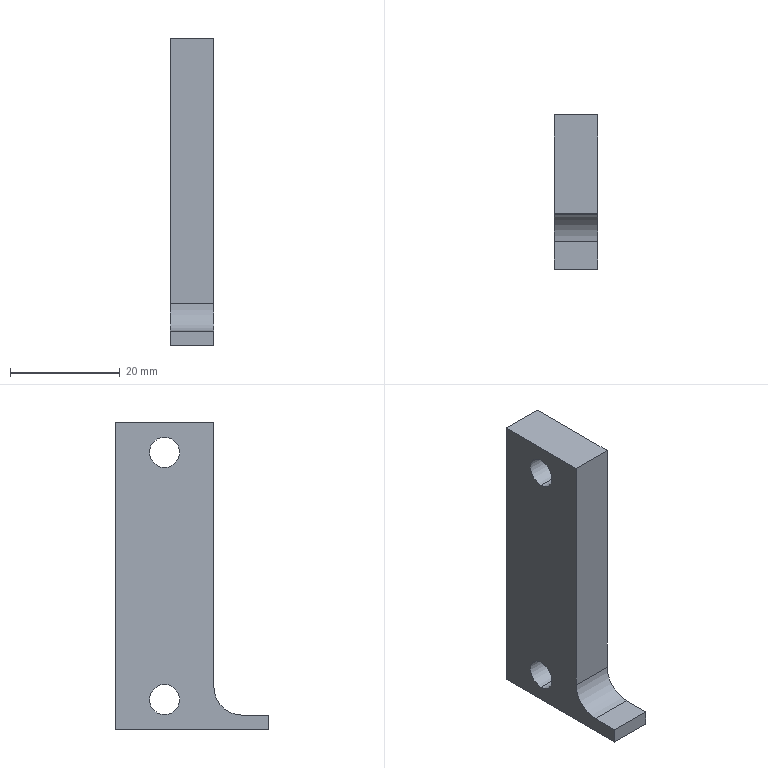Part | NX | 1 solid | 13 faces | box 8 x 28 x 56 mm | volume 7943 mm3 | plane 8 | cylinder 5 | commonest cylinder face diameters 5.5 x4 10 x1
STEP:
#1=CARTESIAN_POINT('',(2319.5,254.4,-75.2));
#2=VERTEX_POINT('',#1);
#3=CARTESIAN_POINT('',(2319.5,226.4,-75.2));
#4=VERTEX_POINT('',#3);
#5=CARTESIAN_POINT('',(2319.5,246.574,-75.2));
#6=DIRECTION('',(0.,-1.,0.));
#7=VECTOR('',#6,1000.);
#8=LINE('',#5,#7);
#9=EDGE_CURVE('',#2,#4,#8,.T.);
#10=ORIENTED_EDGE('',*,*,#9,.F.);
#11=CARTESIAN_POINT('',(2327.5,254.4,-75.2));
#12=VERTEX_POINT('',#11);
#13=CARTESIAN_POINT('',(2321.5,254.4,-75.2));
#14=DIRECTION('',(1.,0.,0.));
#15=VECTOR('',#14,1000.);
#16=LINE('',#13,#15);
#17=EDGE_CURVE('',#2,#12,#16,.T.);
#18=ORIENTED_EDGE('',*,*,#17,.T.);
#19=CARTESIAN_POINT('',(2327.5,226.4,-75.2));
#20=VERTEX_POINT('',#19);
#21=CARTESIAN_POINT('',(2327.5,246.574,-75.2));
#22=DIRECTION('',(0.,1.,0.));
#23=VECTOR('',#22,1000.);
#24=LINE('',#21,#23);
#25=EDGE_CURVE('',#20,#12,#24,.T.);
#26=ORIENTED_EDGE('',*,*,#25,.F.);
#27=CARTESIAN_POINT('',(2321.5,226.4,-75.2));
#28=DIRECTION('',(-1.,0.,0.));
#29=VECTOR('',#28,1000.);
#30=LINE('',#27,#29);
#31=EDGE_CURVE('',#20,#4,#30,.T.);
#32=ORIENTED_EDGE('',*,*,#31,.T.);
#33=EDGE_LOOP('',(#10,#18,#26,#32));
#34=FACE_BOUND('',#33,.T.);
#35=CARTESIAN_POINT('',(2321.5,254.4,-75.2));
#36=DIRECTION('',(0.,0.,-1.));
#37=DIRECTION('',(-1.,0.,0.));
#38=AXIS2_PLACEMENT_3D('',#35,#36,#37);
#39=PLANE('',#38);
#40=ADVANCED_FACE('',(#34),#39,.T.);
#41=CARTESIAN_POINT('',(2319.5,254.4,-19.2));
#42=VERTEX_POINT('',#41);
#43=CARTESIAN_POINT('',(2319.5,254.4,-45.265));
#44=DIRECTION('',(0.,0.,-1.));
#45=VECTOR('',#44,1000.);
#46=LINE('',#43,#45);
#47=EDGE_CURVE('',#42,#2,#46,.T.);
#48=ORIENTED_EDGE('',*,*,#47,.F.);
#49=CARTESIAN_POINT('',(2327.5,254.4,-19.2));
#50=VERTEX_POINT('',#49);
#51=CARTESIAN_POINT('',(2321.5,254.4,-19.2));
#52=DIRECTION('',(1.,0.,0.));
#53=VECTOR('',#52,1000.);
#54=LINE('',#51,#53);
#55=EDGE_CURVE('',#42,#50,#54,.T.);
#56=ORIENTED_EDGE('',*,*,#55,.T.);
#57=CARTESIAN_POINT('',(2327.5,254.4,-75.2));
#58=DIRECTION('',(0.,0.,1.));
#59=VECTOR('',#58,1000.);
#60=LINE('',#57,#59);
#61=EDGE_CURVE('',#12,#50,#60,.T.);
#62=ORIENTED_EDGE('',*,*,#61,.F.);
#63=ORIENTED_EDGE('',*,*,#17,.F.);
#64=EDGE_LOOP('',(#48,#56,#62,#63));
#65=FACE_BOUND('',#64,.T.);
#66=CARTESIAN_POINT('',(2321.5,254.4,-19.2));
#67=DIRECTION('',(0.,1.,0.));
#68=DIRECTION('',(1.,0.,0.));
#69=AXIS2_PLACEMENT_3D('',#66,#67,#68);
#70=PLANE('',#69);
#71=ADVANCED_FACE('',(#65),#70,.T.);
#72=CARTESIAN_POINT('',(2319.5,236.4,-19.2));
#73=VERTEX_POINT('',#72);
#74=CARTESIAN_POINT('',(2319.5,246.574,-19.2));
#75=DIRECTION('',(0.,1.,0.));
#76=VECTOR('',#75,1000.);
#77=LINE('',#74,#76);
#78=EDGE_CURVE('',#73,#42,#77,.T.);
#79=ORIENTED_EDGE('',*,*,#78,.F.);
#80=CARTESIAN_POINT('',(2327.5,236.4,-19.2));
#81=VERTEX_POINT('',#80);
#82=CARTESIAN_POINT('',(2321.5,236.4,-19.2));
#83=DIRECTION('',(1.,0.,0.));
#84=VECTOR('',#83,1000.);
#85=LINE('',#82,#84);
#86=EDGE_CURVE('',#73,#81,#85,.T.);
#87=ORIENTED_EDGE('',*,*,#86,.T.);
#88=CARTESIAN_POINT('',(2327.5,254.4,-19.2));
#89=DIRECTION('',(0.,-1.,0.));
#90=VECTOR('',#89,1000.);
#91=LINE('',#88,#90);
#92=EDGE_CURVE('',#50,#81,#91,.T.);
#93=ORIENTED_EDGE('',*,*,#92,.F.);
#94=ORIENTED_EDGE('',*,*,#55,.F.);
#95=EDGE_LOOP('',(#79,#87,#93,#94));
#96=FACE_BOUND('',#95,.T.);
#97=CARTESIAN_POINT('',(2321.5,236.4,-19.2));
#98=DIRECTION('',(0.,0.,1.));
#99=DIRECTION('',(1.,0.,0.));
#100=AXIS2_PLACEMENT_3D('',#97,#98,#99);
#101=PLANE('',#100);
#102=ADVANCED_FACE('',(#96),#101,.T.);
#103=CARTESIAN_POINT('',(2327.5,236.4,-67.5));
#104=VERTEX_POINT('',#103);
#105=CARTESIAN_POINT('',(2319.5,236.4,-67.5));
#106=VERTEX_POINT('',#105);
#107=CARTESIAN_POINT('',(2321.5,236.4,-67.5));
#108=DIRECTION('',(-1.,0.,0.));
#109=VECTOR('',#108,1000.);
#110=LINE('',#107,#109);
#111=EDGE_CURVE('',#104,#106,#110,.T.);
#112=ORIENTED_EDGE('',*,*,#111,.F.);
#113=CARTESIAN_POINT('',(2327.5,236.4,-45.265));
#114=DIRECTION('',(0.,0.,-1.));
#115=VECTOR('',#114,1000.);
#116=LINE('',#113,#115);
#117=EDGE_CURVE('',#81,#104,#116,.T.);
#118=ORIENTED_EDGE('',*,*,#117,.F.);
#119=ORIENTED_EDGE('',*,*,#86,.F.);
#120=CARTESIAN_POINT('',(2319.5,236.4,-45.265));
#121=DIRECTION('',(0.,0.,1.));
#122=VECTOR('',#121,1000.);
#123=LINE('',#120,#122);
#124=EDGE_CURVE('',#106,#73,#123,.T.);
#125=ORIENTED_EDGE('',*,*,#124,.F.);
#126=EDGE_LOOP('',(#112,#118,#119,#125));
#127=FACE_BOUND('',#126,.T.);
#128=CARTESIAN_POINT('',(2321.5,236.4,-75.2));
#129=DIRECTION('',(0.,-1.,0.));
#130=DIRECTION('',(0.,0.,-1.));
#131=AXIS2_PLACEMENT_3D('',#128,#129,#130);
#132=PLANE('',#131);
#133=ADVANCED_FACE('',(#127),#132,.T.);
#134=CARTESIAN_POINT('',(2327.5,226.4,-72.5));
#135=VERTEX_POINT('',#134);
#136=CARTESIAN_POINT('',(2327.5,226.4,-45.265));
#137=DIRECTION('',(0.,0.,-1.));
#138=VECTOR('',#137,1000.);
#139=LINE('',#136,#138);
#140=EDGE_CURVE('',#135,#20,#139,.T.);
#141=ORIENTED_EDGE('',*,*,#140,.F.);
#142=CARTESIAN_POINT('',(2319.5,226.4,-72.5));
#143=VERTEX_POINT('',#142);
#144=CARTESIAN_POINT('',(2321.5,226.4,-72.5));
#145=DIRECTION('',(-1.,0.,0.));
#146=VECTOR('',#145,1000.);
#147=LINE('',#144,#146);
#148=EDGE_CURVE('',#135,#143,#147,.T.);
#149=ORIENTED_EDGE('',*,*,#148,.T.);
#150=CARTESIAN_POINT('',(2319.5,226.4,-45.265));
#151=DIRECTION('',(0.,0.,-1.));
#152=VECTOR('',#151,1000.);
#153=LINE('',#150,#152);
#154=EDGE_CURVE('',#143,#4,#153,.T.);
#155=ORIENTED_EDGE('',*,*,#154,.T.);
#156=ORIENTED_EDGE('',*,*,#31,.F.);
#157=EDGE_LOOP('',(#141,#149,#155,#156));
#158=FACE_BOUND('',#157,.T.);
#159=CARTESIAN_POINT('',(2325.077,226.4,-68.526));
#160=DIRECTION('',(0.,-1.,0.));
#161=DIRECTION('',(0.,0.,-1.));
#162=AXIS2_PLACEMENT_3D('',#159,#160,#161);
#163=PLANE('',#162);
#164=ADVANCED_FACE('',(#158),#163,.T.);
#165=CARTESIAN_POINT('',(2327.5,231.4,-72.5));
#166=VERTEX_POINT('',#165);
#167=CARTESIAN_POINT('',(2319.5,231.4,-72.5));
#168=VERTEX_POINT('',#167);
#169=CARTESIAN_POINT('',(2321.5,231.4,-72.5));
#170=DIRECTION('',(-1.,0.,0.));
#171=VECTOR('',#170,1000.);
#172=LINE('',#169,#171);
#173=EDGE_CURVE('',#166,#168,#172,.T.);
#174=ORIENTED_EDGE('',*,*,#173,.T.);
#175=CARTESIAN_POINT('',(2319.5,246.574,-72.5));
#176=DIRECTION('',(0.,-1.,0.));
#177=VECTOR('',#176,1000.);
#178=LINE('',#175,#177);
#179=EDGE_CURVE('',#168,#143,#178,.T.);
#180=ORIENTED_EDGE('',*,*,#179,.T.);
#181=ORIENTED_EDGE('',*,*,#148,.F.);
#182=CARTESIAN_POINT('',(2327.5,246.574,-72.5));
#183=DIRECTION('',(0.,-1.,0.));
#184=VECTOR('',#183,1000.);
#185=LINE('',#182,#184);
#186=EDGE_CURVE('',#166,#135,#185,.T.);
#187=ORIENTED_EDGE('',*,*,#186,.F.);
#188=EDGE_LOOP('',(#174,#180,#181,#187));
#189=FACE_BOUND('',#188,.T.);
#190=CARTESIAN_POINT('',(2321.5,236.4,-72.5));
#191=DIRECTION('',(0.,0.,1.));
#192=DIRECTION('',(1.,0.,0.));
#193=AXIS2_PLACEMENT_3D('',#190,#191,#192);
#194=PLANE('',#193);
#195=ADVANCED_FACE('',(#189),#194,.T.);
#196=ORIENTED_EDGE('',*,*,#111,.T.);
#197=CARTESIAN_POINT('',(2319.5,231.4,-67.5));
#198=DIRECTION('',(-1.,0.,0.));
#199=DIRECTION('',(0.,0.,-1.));
#200=AXIS2_PLACEMENT_3D('',#197,#198,#199);
#201=CIRCLE('',#200,5.);
#202=EDGE_CURVE('',#106,#168,#201,.T.);
#203=ORIENTED_EDGE('',*,*,#202,.T.);
#204=ORIENTED_EDGE('',*,*,#173,.F.);
#205=CARTESIAN_POINT('',(2327.5,231.4,-67.5));
#206=DIRECTION('',(-1.,0.,0.));
#207=DIRECTION('',(0.,0.,-1.));
#208=AXIS2_PLACEMENT_3D('',#205,#206,#207);
#209=CIRCLE('',#208,5.);
#210=EDGE_CURVE('',#104,#166,#209,.T.);
#211=ORIENTED_EDGE('',*,*,#210,.F.);
#212=EDGE_LOOP('',(#196,#203,#204,#211));
#213=FACE_BOUND('',#212,.T.);
#214=CARTESIAN_POINT('',(2321.5,231.4,-67.5));
#215=DIRECTION('',(-1.,0.,0.));
#216=DIRECTION('',(0.,0.,-1.));
#217=AXIS2_PLACEMENT_3D('',#214,#215,#216);
#218=CYLINDRICAL_SURFACE('',#217,5.);
#219=ADVANCED_FACE('',(#213),#218,.F.);
#220=ORIENTED_EDGE('',*,*,#61,.T.);
#221=ORIENTED_EDGE('',*,*,#92,.T.);
#222=ORIENTED_EDGE('',*,*,#117,.T.);
#223=ORIENTED_EDGE('',*,*,#210,.T.);
#224=ORIENTED_EDGE('',*,*,#186,.T.);
#225=ORIENTED_EDGE('',*,*,#140,.T.);
#226=ORIENTED_EDGE('',*,*,#25,.T.);
#227=EDGE_LOOP('',(#220,#221,#222,#223,#224,#225,#226));
#228=FACE_BOUND('',#227,.T.);
#229=CARTESIAN_POINT('',(2327.5,245.4,-66.95));
#230=VERTEX_POINT('',#229);
#231=CARTESIAN_POINT('',(2327.5,245.4,-72.45));
#232=VERTEX_POINT('',#231);
#233=CARTESIAN_POINT('',(2327.5,245.4,-69.7));
#234=DIRECTION('',(1.,0.,0.));
#235=DIRECTION('',(0.,0.,-1.));
#236=AXIS2_PLACEMENT_3D('',#233,#234,#235);
#237=CIRCLE('',#236,2.75);
#238=EDGE_CURVE('',#230,#232,#237,.T.);
#239=ORIENTED_EDGE('',*,*,#238,.F.);
#240=CARTESIAN_POINT('',(2327.5,245.4,-69.7));
#241=DIRECTION('',(1.,0.,0.));
#242=DIRECTION('',(0.,0.,-1.));
#243=AXIS2_PLACEMENT_3D('',#240,#241,#242);
#244=CIRCLE('',#243,2.75);
#245=EDGE_CURVE('',#232,#230,#244,.T.);
#246=ORIENTED_EDGE('',*,*,#245,.F.);
#247=EDGE_LOOP('',(#239,#246));
#248=FACE_BOUND('',#247,.T.);
#249=CARTESIAN_POINT('',(2327.5,245.4,-21.95));
#250=VERTEX_POINT('',#249);
#251=CARTESIAN_POINT('',(2327.5,245.4,-27.45));
#252=VERTEX_POINT('',#251);
#253=CARTESIAN_POINT('',(2327.5,245.4,-24.7));
#254=DIRECTION('',(1.,0.,0.));
#255=DIRECTION('',(0.,0.,-1.));
#256=AXIS2_PLACEMENT_3D('',#253,#254,#255);
#257=CIRCLE('',#256,2.75);
#258=EDGE_CURVE('',#250,#252,#257,.T.);
#259=ORIENTED_EDGE('',*,*,#258,.F.);
#260=CARTESIAN_POINT('',(2327.5,245.4,-24.7));
#261=DIRECTION('',(1.,0.,0.));
#262=DIRECTION('',(0.,0.,-1.));
#263=AXIS2_PLACEMENT_3D('',#260,#261,#262);
#264=CIRCLE('',#263,2.75);
#265=EDGE_CURVE('',#252,#250,#264,.T.);
#266=ORIENTED_EDGE('',*,*,#265,.F.);
#267=EDGE_LOOP('',(#259,#266));
#268=FACE_BOUND('',#267,.T.);
#269=CARTESIAN_POINT('',(2327.5,246.574,-45.265));
#270=DIRECTION('',(1.,0.,0.));
#271=DIRECTION('',(0.,1.,0.));
#272=AXIS2_PLACEMENT_3D('',#269,#270,#271);
#273=PLANE('',#272);
#274=ADVANCED_FACE('',(#228,#248,#268),#273,.T.);
#275=ORIENTED_EDGE('',*,*,#258,.T.);
#276=CARTESIAN_POINT('',(2319.5,245.4,-27.45));
#277=VERTEX_POINT('',#276);
#278=CARTESIAN_POINT('',(2320.9,245.4,-27.45));
#279=DIRECTION('',(1.,0.,0.));
#280=VECTOR('',#279,1000.);
#281=LINE('',#278,#280);
#282=EDGE_CURVE('',#252,#277,#281,.F.);
#283=ORIENTED_EDGE('',*,*,#282,.T.);
#284=CARTESIAN_POINT('',(2319.5,245.4,-21.95));
#285=VERTEX_POINT('',#284);
#286=CARTESIAN_POINT('',(2319.5,245.4,-24.7));
#287=DIRECTION('',(1.,0.,0.));
#288=DIRECTION('',(0.,0.,-1.));
#289=AXIS2_PLACEMENT_3D('',#286,#287,#288);
#290=CIRCLE('',#289,2.75);
#291=EDGE_CURVE('',#285,#277,#290,.T.);
#292=ORIENTED_EDGE('',*,*,#291,.F.);
#293=CARTESIAN_POINT('',(2320.9,245.4,-21.95));
#294=DIRECTION('',(1.,0.,0.));
#295=VECTOR('',#294,1000.);
#296=LINE('',#293,#295);
#297=EDGE_CURVE('',#250,#285,#296,.F.);
#298=ORIENTED_EDGE('',*,*,#297,.F.);
#299=EDGE_LOOP('',(#275,#283,#292,#298));
#300=FACE_BOUND('',#299,.T.);
#301=CARTESIAN_POINT('',(2320.9,245.4,-24.7));
#302=DIRECTION('',(1.,0.,0.));
#303=DIRECTION('',(0.,0.,-1.));
#304=AXIS2_PLACEMENT_3D('',#301,#302,#303);
#305=CYLINDRICAL_SURFACE('',#304,2.75);
#306=ADVANCED_FACE('',(#300),#305,.F.);
#307=CARTESIAN_POINT('',(2319.5,245.4,-66.95));
#308=VERTEX_POINT('',#307);
#309=CARTESIAN_POINT('',(2319.5,245.4,-72.45));
#310=VERTEX_POINT('',#309);
#311=CARTESIAN_POINT('',(2319.5,245.4,-69.7));
#312=DIRECTION('',(1.,0.,0.));
#313=DIRECTION('',(0.,0.,-1.));
#314=AXIS2_PLACEMENT_3D('',#311,#312,#313);
#315=CIRCLE('',#314,2.75);
#316=EDGE_CURVE('',#308,#310,#315,.T.);
#317=ORIENTED_EDGE('',*,*,#316,.F.);
#318=CARTESIAN_POINT('',(2320.9,245.4,-66.95));
#319=DIRECTION('',(1.,0.,0.));
#320=VECTOR('',#319,1000.);
#321=LINE('',#318,#320);
#322=EDGE_CURVE('',#230,#308,#321,.F.);
#323=ORIENTED_EDGE('',*,*,#322,.F.);
#324=ORIENTED_EDGE('',*,*,#238,.T.);
#325=CARTESIAN_POINT('',(2320.9,245.4,-72.45));
#326=DIRECTION('',(1.,0.,0.));
#327=VECTOR('',#326,1000.);
#328=LINE('',#325,#327);
#329=EDGE_CURVE('',#232,#310,#328,.F.);
#330=ORIENTED_EDGE('',*,*,#329,.T.);
#331=EDGE_LOOP('',(#317,#323,#324,#330));
#332=FACE_BOUND('',#331,.T.);
#333=CARTESIAN_POINT('',(2320.9,245.4,-69.7));
#334=DIRECTION('',(1.,0.,0.));
#335=DIRECTION('',(0.,0.,-1.));
#336=AXIS2_PLACEMENT_3D('',#333,#334,#335);
#337=CYLINDRICAL_SURFACE('',#336,2.75);
#338=ADVANCED_FACE('',(#332),#337,.F.);
#339=ORIENTED_EDGE('',*,*,#9,.T.);
#340=ORIENTED_EDGE('',*,*,#154,.F.);
#341=ORIENTED_EDGE('',*,*,#179,.F.);
#342=ORIENTED_EDGE('',*,*,#202,.F.);
#343=ORIENTED_EDGE('',*,*,#124,.T.);
#344=ORIENTED_EDGE('',*,*,#78,.T.);
#345=ORIENTED_EDGE('',*,*,#47,.T.);
#346=EDGE_LOOP('',(#339,#340,#341,#342,#343,#344,#345));
#347=FACE_BOUND('',#346,.T.);
#348=CARTESIAN_POINT('',(2319.5,245.4,-24.7));
#349=DIRECTION('',(1.,0.,0.));
#350=DIRECTION('',(0.,0.,-1.));
#351=AXIS2_PLACEMENT_3D('',#348,#349,#350);
#352=CIRCLE('',#351,2.75);
#353=EDGE_CURVE('',#277,#285,#352,.T.);
#354=ORIENTED_EDGE('',*,*,#353,.T.);
#355=ORIENTED_EDGE('',*,*,#291,.T.);
#356=EDGE_LOOP('',(#354,#355));
#357=FACE_BOUND('',#356,.T.);
#358=ORIENTED_EDGE('',*,*,#316,.T.);
#359=CARTESIAN_POINT('',(2319.5,245.4,-69.7));
#360=DIRECTION('',(1.,0.,0.));
#361=DIRECTION('',(0.,0.,-1.));
#362=AXIS2_PLACEMENT_3D('',#359,#360,#361);
#363=CIRCLE('',#362,2.75);
#364=EDGE_CURVE('',#310,#308,#363,.T.);
#365=ORIENTED_EDGE('',*,*,#364,.T.);
#366=EDGE_LOOP('',(#358,#365));
#367=FACE_BOUND('',#366,.T.);
#368=CARTESIAN_POINT('',(2319.5,246.574,-45.265));
#369=DIRECTION('',(1.,0.,0.));
#370=DIRECTION('',(0.,1.,0.));
#371=AXIS2_PLACEMENT_3D('',#368,#369,#370);
#372=PLANE('',#371);
#373=ADVANCED_FACE('',(#347,#357,#367),#372,.F.);
#374=ORIENTED_EDGE('',*,*,#353,.F.);
#375=ORIENTED_EDGE('',*,*,#282,.F.);
#376=ORIENTED_EDGE('',*,*,#265,.T.);
#377=ORIENTED_EDGE('',*,*,#297,.T.);
#378=EDGE_LOOP('',(#374,#375,#376,#377));
#379=FACE_BOUND('',#378,.T.);
#380=CARTESIAN_POINT('',(2320.9,245.4,-24.7));
#381=DIRECTION('',(1.,0.,0.));
#382=DIRECTION('',(0.,0.,-1.));
#383=AXIS2_PLACEMENT_3D('',#380,#381,#382);
#384=CYLINDRICAL_SURFACE('',#383,2.75);
#385=ADVANCED_FACE('',(#379),#384,.F.);
#386=ORIENTED_EDGE('',*,*,#329,.F.);
#387=ORIENTED_EDGE('',*,*,#245,.T.);
#388=ORIENTED_EDGE('',*,*,#322,.T.);
#389=ORIENTED_EDGE('',*,*,#364,.F.);
#390=EDGE_LOOP('',(#386,#387,#388,#389));
#391=FACE_BOUND('',#390,.T.);
#392=CARTESIAN_POINT('',(2320.9,245.4,-69.7));
#393=DIRECTION('',(1.,0.,0.));
#394=DIRECTION('',(0.,0.,-1.));
#395=AXIS2_PLACEMENT_3D('',#392,#393,#394);
#396=CYLINDRICAL_SURFACE('',#395,2.75);
#397=ADVANCED_FACE('',(#391),#396,.F.);
#398=CLOSED_SHELL('',(#40,#71,#102,#133,#164,#195,#219,#274,#306,#338,#373,#385,#397));
#399=MANIFOLD_SOLID_BREP('',#398);
#400=(LENGTH_UNIT()NAMED_UNIT(*)SI_UNIT(.MILLI.,.METRE.));
#401=UNCERTAINTY_MEASURE_WITH_UNIT(LENGTH_MEASURE(0.00001),#400,'','');
#402=(NAMED_UNIT(*)PLANE_ANGLE_UNIT()SI_UNIT($,.RADIAN.));
#403=(NAMED_UNIT(*)SI_UNIT($,.STERADIAN.)SOLID_ANGLE_UNIT());
#404=(GEOMETRIC_REPRESENTATION_CONTEXT(3)GLOBAL_UNCERTAINTY_ASSIGNED_CONTEXT((#401))GLOBAL_UNIT_ASSIGNED_CONTEXT((#400,#402,#403))REPRESENTATION_CONTEXT('',''));
#405=ADVANCED_BREP_SHAPE_REPRESENTATION('',(#399),#404);